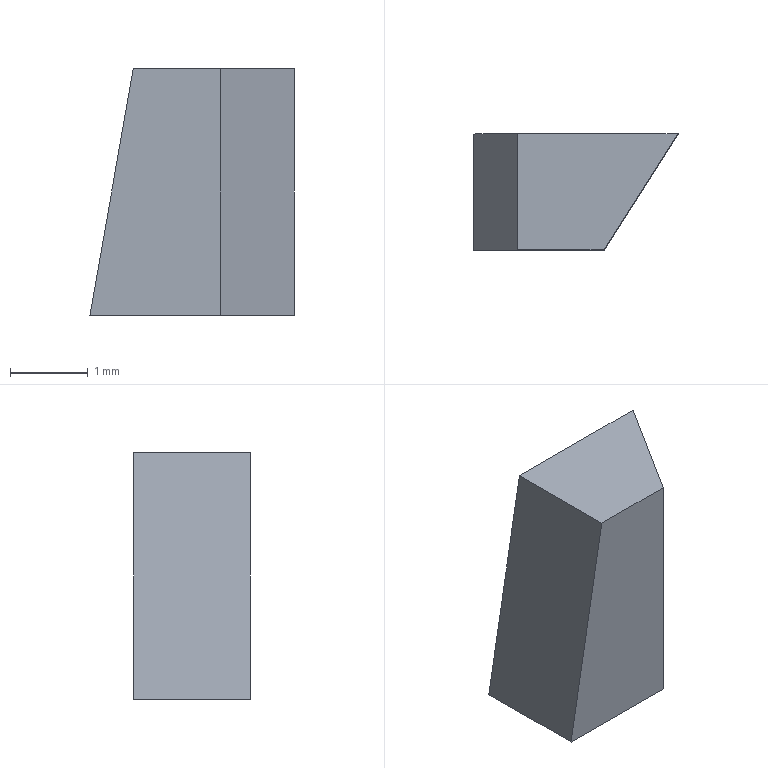Part | SolidWorks | features Extrusion 1, ICE 1 | 1 solid | 6 faces | box 2.63 x 1.5 x 3.175 mm | volume 8.931 mm3 | plane 6
STEP:
#1=CARTESIAN_POINT('',(-6.086,5.,0.));
#2=VERTEX_POINT('',#1);
#3=CARTESIAN_POINT('',(-5.528,5.,3.175));
#4=VERTEX_POINT('',#3);
#5=CARTESIAN_POINT('',(-6.086,5.,0.));
#6=DIRECTION('',(0.1731,0.,0.9849));
#7=VECTOR('',#6,1000.);
#8=LINE('',#5,#7);
#9=EDGE_CURVE('',#2,#4,#8,.T.);
#10=ORIENTED_EDGE('',*,*,#9,.F.);
#11=CARTESIAN_POINT('',(-4.408,5.,0.));
#12=VERTEX_POINT('',#11);
#13=CARTESIAN_POINT('',(-4.408,5.,0.));
#14=DIRECTION('',(-1.,0.,0.));
#15=VECTOR('',#14,1000.);
#16=LINE('',#13,#15);
#17=EDGE_CURVE('',#12,#2,#16,.T.);
#18=ORIENTED_EDGE('',*,*,#17,.F.);
#19=CARTESIAN_POINT('',(-4.408,5.,3.175));
#20=VERTEX_POINT('',#19);
#21=CARTESIAN_POINT('',(-4.408,5.,3.175));
#22=DIRECTION('',(0.,0.,-1.));
#23=VECTOR('',#22,1000.);
#24=LINE('',#21,#23);
#25=EDGE_CURVE('',#20,#12,#24,.T.);
#26=ORIENTED_EDGE('',*,*,#25,.F.);
#27=CARTESIAN_POINT('',(-4.408,5.,3.175));
#28=DIRECTION('',(-1.,0.,0.));
#29=VECTOR('',#28,1000.);
#30=LINE('',#27,#29);
#31=EDGE_CURVE('',#20,#4,#30,.T.);
#32=ORIENTED_EDGE('',*,*,#31,.T.);
#33=EDGE_LOOP('',(#10,#18,#26,#32));
#34=FACE_OUTER_BOUND('',#33,.T.);
#35=CARTESIAN_POINT('',(-4.408,5.,3.175));
#36=DIRECTION('',(0.,-1.,0.));
#37=DIRECTION('',(1.,0.,0.));
#38=AXIS2_PLACEMENT_3D('',#35,#36,#37);
#39=PLANE('',#38);
#40=ADVANCED_FACE('',(#34),#39,.T.);
#41=CARTESIAN_POINT('',(-3.455,6.5,0.));
#42=VERTEX_POINT('',#41);
#43=CARTESIAN_POINT('',(-3.455,6.5,0.));
#44=DIRECTION('',(-0.5361,-0.8442,0.));
#45=VECTOR('',#44,1000.);
#46=LINE('',#43,#45);
#47=EDGE_CURVE('',#42,#12,#46,.T.);
#48=ORIENTED_EDGE('',*,*,#47,.F.);
#49=CARTESIAN_POINT('',(-3.455,6.5,3.175));
#50=VERTEX_POINT('',#49);
#51=CARTESIAN_POINT('',(-3.455,6.5,3.175));
#52=DIRECTION('',(0.,0.,-1.));
#53=VECTOR('',#52,1000.);
#54=LINE('',#51,#53);
#55=EDGE_CURVE('',#50,#42,#54,.T.);
#56=ORIENTED_EDGE('',*,*,#55,.F.);
#57=CARTESIAN_POINT('',(-3.455,6.5,3.175));
#58=DIRECTION('',(-0.5361,-0.8442,0.));
#59=VECTOR('',#58,1000.);
#60=LINE('',#57,#59);
#61=EDGE_CURVE('',#50,#20,#60,.T.);
#62=ORIENTED_EDGE('',*,*,#61,.T.);
#63=ORIENTED_EDGE('',*,*,#25,.T.);
#64=EDGE_LOOP('',(#48,#56,#62,#63));
#65=FACE_OUTER_BOUND('',#64,.T.);
#66=CARTESIAN_POINT('',(-3.455,6.5,3.175));
#67=DIRECTION('',(0.8442,-0.5361,0.));
#68=DIRECTION('',(0.5361,0.8442,0.));
#69=AXIS2_PLACEMENT_3D('',#66,#67,#68);
#70=PLANE('',#69);
#71=ADVANCED_FACE('',(#65),#70,.T.);
#72=CARTESIAN_POINT('',(-5.528,6.5,3.175));
#73=VERTEX_POINT('',#72);
#74=CARTESIAN_POINT('',(-6.086,6.5,0.));
#75=VERTEX_POINT('',#74);
#76=CARTESIAN_POINT('',(-5.584,6.5,2.854));
#77=DIRECTION('',(-0.1731,0.,-0.9849));
#78=VECTOR('',#77,1000.);
#79=LINE('',#76,#78);
#80=EDGE_CURVE('',#73,#75,#79,.T.);
#81=ORIENTED_EDGE('',*,*,#80,.F.);
#82=CARTESIAN_POINT('',(-7.408,6.5,3.175));
#83=DIRECTION('',(1.,0.,0.));
#84=VECTOR('',#83,1000.);
#85=LINE('',#82,#84);
#86=EDGE_CURVE('',#73,#50,#85,.T.);
#87=ORIENTED_EDGE('',*,*,#86,.T.);
#88=ORIENTED_EDGE('',*,*,#55,.T.);
#89=CARTESIAN_POINT('',(-7.408,6.5,0.));
#90=DIRECTION('',(1.,0.,0.));
#91=VECTOR('',#90,1000.);
#92=LINE('',#89,#91);
#93=EDGE_CURVE('',#75,#42,#92,.T.);
#94=ORIENTED_EDGE('',*,*,#93,.F.);
#95=EDGE_LOOP('',(#81,#87,#88,#94));
#96=FACE_OUTER_BOUND('',#95,.T.);
#97=CARTESIAN_POINT('',(-7.408,6.5,3.175));
#98=DIRECTION('',(0.,1.,0.));
#99=DIRECTION('',(-1.,0.,0.));
#100=AXIS2_PLACEMENT_3D('',#97,#98,#99);
#101=PLANE('',#100);
#102=ADVANCED_FACE('',(#96),#101,.T.);
#103=ORIENTED_EDGE('',*,*,#86,.F.);
#104=CARTESIAN_POINT('',(-5.528,8.175,3.175));
#105=DIRECTION('',(0.,-1.,0.));
#106=VECTOR('',#105,1000.);
#107=LINE('',#104,#106);
#108=EDGE_CURVE('',#73,#4,#107,.T.);
#109=ORIENTED_EDGE('',*,*,#108,.T.);
#110=ORIENTED_EDGE('',*,*,#31,.F.);
#111=ORIENTED_EDGE('',*,*,#61,.F.);
#112=EDGE_LOOP('',(#103,#109,#110,#111));
#113=FACE_OUTER_BOUND('',#112,.T.);
#114=CARTESIAN_POINT('',(0.,0.,3.175));
#115=DIRECTION('',(0.,0.,-1.));
#116=DIRECTION('',(-1.,0.,0.));
#117=AXIS2_PLACEMENT_3D('',#114,#115,#116);
#118=PLANE('',#117);
#119=ADVANCED_FACE('',(#113),#118,.F.);
#120=CARTESIAN_POINT('',(-6.086,0.,0.));
#121=DIRECTION('',(0.,-1.,0.));
#122=VECTOR('',#121,1000.);
#123=LINE('',#120,#122);
#124=EDGE_CURVE('',#75,#2,#123,.T.);
#125=ORIENTED_EDGE('',*,*,#124,.F.);
#126=ORIENTED_EDGE('',*,*,#93,.T.);
#127=ORIENTED_EDGE('',*,*,#47,.T.);
#128=ORIENTED_EDGE('',*,*,#17,.T.);
#129=EDGE_LOOP('',(#125,#126,#127,#128));
#130=FACE_OUTER_BOUND('',#129,.T.);
#131=CARTESIAN_POINT('',(0.,0.,0.));
#132=DIRECTION('',(0.,0.,-1.));
#133=DIRECTION('',(-1.,0.,0.));
#134=AXIS2_PLACEMENT_3D('',#131,#132,#133);
#135=PLANE('',#134);
#136=ADVANCED_FACE('',(#130),#135,.T.);
#137=ORIENTED_EDGE('',*,*,#80,.T.);
#138=ORIENTED_EDGE('',*,*,#124,.T.);
#139=ORIENTED_EDGE('',*,*,#9,.T.);
#140=ORIENTED_EDGE('',*,*,#108,.F.);
#141=EDGE_LOOP('',(#137,#138,#139,#140));
#142=FACE_OUTER_BOUND('',#141,.T.);
#143=CARTESIAN_POINT('',(-6.086,8.175,0.));
#144=DIRECTION('',(0.9849,0.,-0.1731));
#145=DIRECTION('',(-0.1731,0.,-0.9849));
#146=AXIS2_PLACEMENT_3D('',#143,#144,#145);
#147=PLANE('',#146);
#148=ADVANCED_FACE('',(#142),#147,.F.);
#149=CLOSED_SHELL('',(#40,#71,#102,#119,#136,#148));
#150=MANIFOLD_SOLID_BREP('',#149);
#151=CARTESIAN_POINT('',(0.,0.,0.));
#152=DIRECTION('',(0.,0.,1.));
#153=DIRECTION('',(1.,0.,0.));
#154=AXIS2_PLACEMENT_3D('',#151,#152,#153);
#155=(LENGTH_UNIT()NAMED_UNIT(*)SI_UNIT(.MILLI.,.METRE.));
#156=UNCERTAINTY_MEASURE_WITH_UNIT(LENGTH_MEASURE(0.00001),#155,'','');
#157=(NAMED_UNIT(*)PLANE_ANGLE_UNIT()SI_UNIT($,.RADIAN.));
#158=(NAMED_UNIT(*)SI_UNIT($,.STERADIAN.)SOLID_ANGLE_UNIT());
#159=(GEOMETRIC_REPRESENTATION_CONTEXT(3)GLOBAL_UNCERTAINTY_ASSIGNED_CONTEXT((#156))GLOBAL_UNIT_ASSIGNED_CONTEXT((#155,#157,#158))REPRESENTATION_CONTEXT('',''));
#160=ADVANCED_BREP_SHAPE_REPRESENTATION('',(#150,#154),#159);